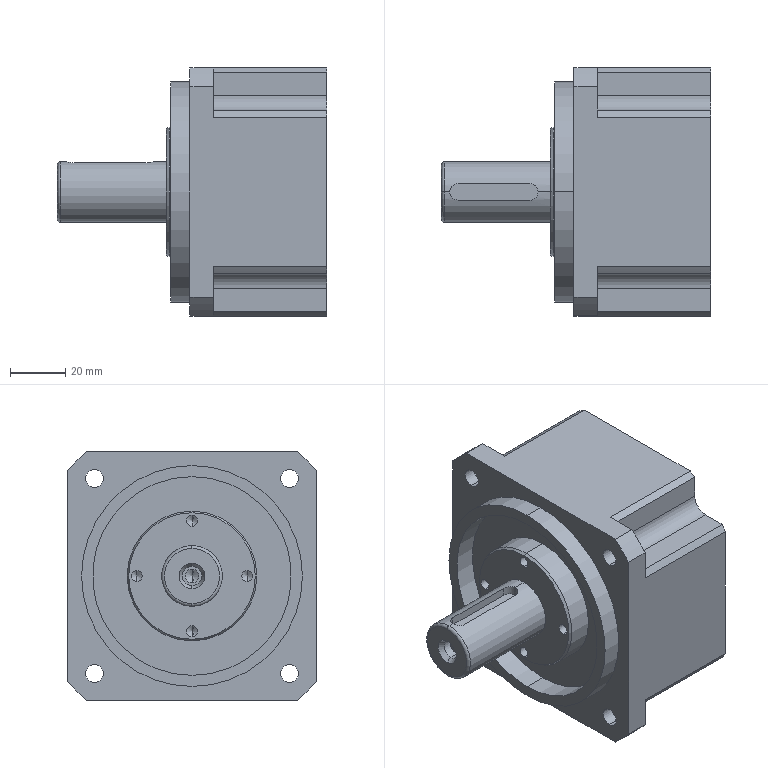Part | SolidWorks | features BaseBody 1 | 1 solid | 92 faces | box 97.5 x 90 x 90 mm | volume 377661 mm3 | cylinder 49 | plane 27 | cone 14 | torus 2 | commonest cylinder face diameters 4 x8 6.5 x8 105 x8 11 x4 118 x4 6 x3